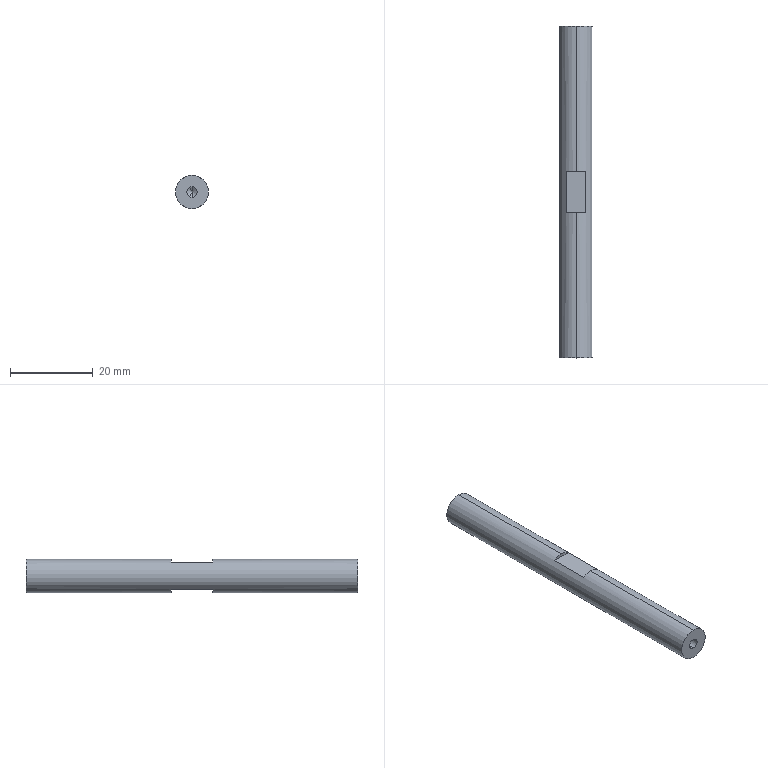Part | STEP file | PN_0039 | 1 solid | 18 faces | box 8 x 80 x 8 mm | volume 3898 mm3 | plane 8 | cylinder 6 | cone 4 | commonest cylinder face diameters 2.5 x4 8 x2
STEP:
#1=CARTESIAN_POINT('',(0.,0.,0.));
#2=DIRECTION('',(0.,0.,1.));
#3=DIRECTION('',(1.,0.,0.));
#4=AXIS2_PLACEMENT_3D('',#1,#2,#3);
#5=CARTESIAN_POINT('',(0.,32.5,1.25));
#6=VERTEX_POINT('',#5);
#7=CARTESIAN_POINT('',(0.,40.,1.25));
#8=VERTEX_POINT('',#7);
#9=CARTESIAN_POINT('',(0.,40.,1.25));
#10=DIRECTION('',(0.,1.,0.));
#11=VECTOR('',#10,1.);
#12=LINE('',#9,#11);
#13=CARTESIAN_POINT('',(0.,40.,0.));
#14=DIRECTION('',(0.,1.,0.));
#15=DIRECTION('',(0.,0.,1.));
#16=AXIS2_PLACEMENT_3D('',#13,#14,#15);
#17=CYLINDRICAL_SURFACE('',#16,1.25);
#18=CARTESIAN_POINT('',(6.283,0.));
#19=DIRECTION('',(0.,1.));
#20=VECTOR('',#19,1.);
#21=LINE('',#18,#20);
#22=(GEOMETRIC_REPRESENTATION_CONTEXT(2)PARAMETRIC_REPRESENTATION_CONTEXT()REPRESENTATION_CONTEXT('',''));
#23=DEFINITIONAL_REPRESENTATION('',(#21),#22);
#24=PCURVE('',#17,#23);
#25=CARTESIAN_POINT('',(0.,40.,0.));
#26=DIRECTION('',(0.,1.,0.));
#27=DIRECTION('',(0.,0.,1.));
#28=AXIS2_PLACEMENT_3D('',#25,#26,#27);
#29=CYLINDRICAL_SURFACE('',#28,1.25);
#30=CARTESIAN_POINT('',(0.,0.));
#31=DIRECTION('',(0.,1.));
#32=VECTOR('',#31,1.);
#33=LINE('',#30,#32);
#34=(GEOMETRIC_REPRESENTATION_CONTEXT(2)PARAMETRIC_REPRESENTATION_CONTEXT()REPRESENTATION_CONTEXT('',''));
#35=DEFINITIONAL_REPRESENTATION('',(#33),#34);
#36=PCURVE('',#29,#35);
#37=SURFACE_CURVE('',#12,(#24,#36),.PCURVE_S1.);
#38=EDGE_CURVE('',#6,#8,#37,.T.);
#39=ORIENTED_EDGE('',*,*,#38,.T.);
#40=CARTESIAN_POINT('',(0.,40.,-1.25));
#41=VERTEX_POINT('',#40);
#42=CARTESIAN_POINT('',(0.,40.,0.));
#43=DIRECTION('',(0.,1.,0.));
#44=DIRECTION('',(0.,0.,1.));
#45=AXIS2_PLACEMENT_3D('',#42,#43,#44);
#46=CIRCLE('',#45,1.25);
#47=CARTESIAN_POINT('',(0.,0.));
#48=DIRECTION('',(1.,0.));
#49=VECTOR('',#48,1.);
#50=LINE('',#47,#49);
#51=(GEOMETRIC_REPRESENTATION_CONTEXT(2)PARAMETRIC_REPRESENTATION_CONTEXT()REPRESENTATION_CONTEXT('',''));
#52=DEFINITIONAL_REPRESENTATION('',(#50),#51);
#53=PCURVE('',#17,#52);
#54=CARTESIAN_POINT('',(0.,40.,0.));
#55=DIRECTION('',(0.,1.,0.));
#56=DIRECTION('',(0.,0.,1.));
#57=AXIS2_PLACEMENT_3D('',#54,#55,#56);
#58=PLANE('',#57);
#59=CARTESIAN_POINT('',(0.,0.));
#60=DIRECTION('',(1.,0.));
#61=AXIS2_PLACEMENT_2D('',#59,#60);
#62=CIRCLE('',#61,1.25);
#63=(GEOMETRIC_REPRESENTATION_CONTEXT(2)PARAMETRIC_REPRESENTATION_CONTEXT()REPRESENTATION_CONTEXT('',''));
#64=DEFINITIONAL_REPRESENTATION('',(#62),#63);
#65=PCURVE('',#58,#64);
#66=SURFACE_CURVE('',#46,(#53,#65),.PCURVE_S1.);
#67=EDGE_CURVE('',#41,#8,#66,.T.);
#68=ORIENTED_EDGE('',*,*,#67,.F.);
#69=CARTESIAN_POINT('',(0.,32.5,-1.25));
#70=VERTEX_POINT('',#69);
#71=CARTESIAN_POINT('',(0.,40.,-1.25));
#72=DIRECTION('',(0.,1.,0.));
#73=VECTOR('',#72,1.);
#74=LINE('',#71,#73);
#75=CARTESIAN_POINT('',(3.142,0.));
#76=DIRECTION('',(0.,1.));
#77=VECTOR('',#76,1.);
#78=LINE('',#75,#77);
#79=(GEOMETRIC_REPRESENTATION_CONTEXT(2)PARAMETRIC_REPRESENTATION_CONTEXT()REPRESENTATION_CONTEXT('',''));
#80=DEFINITIONAL_REPRESENTATION('',(#78),#79);
#81=PCURVE('',#17,#80);
#82=CARTESIAN_POINT('',(3.142,0.));
#83=DIRECTION('',(0.,1.));
#84=VECTOR('',#83,1.);
#85=LINE('',#82,#84);
#86=(GEOMETRIC_REPRESENTATION_CONTEXT(2)PARAMETRIC_REPRESENTATION_CONTEXT()REPRESENTATION_CONTEXT('',''));
#87=DEFINITIONAL_REPRESENTATION('',(#85),#86);
#88=PCURVE('',#29,#87);
#89=SURFACE_CURVE('',#74,(#81,#88),.PCURVE_S1.);
#90=EDGE_CURVE('',#70,#41,#89,.T.);
#91=ORIENTED_EDGE('',*,*,#90,.F.);
#92=CARTESIAN_POINT('',(0.,32.5,0.));
#93=DIRECTION('',(0.,1.,0.));
#94=DIRECTION('',(0.,0.,1.));
#95=AXIS2_PLACEMENT_3D('',#92,#93,#94);
#96=CIRCLE('',#95,1.25);
#97=CARTESIAN_POINT('',(0.,-7.5));
#98=DIRECTION('',(1.,0.));
#99=VECTOR('',#98,1.);
#100=LINE('',#97,#99);
#101=(GEOMETRIC_REPRESENTATION_CONTEXT(2)PARAMETRIC_REPRESENTATION_CONTEXT()REPRESENTATION_CONTEXT('',''));
#102=DEFINITIONAL_REPRESENTATION('',(#100),#101);
#103=PCURVE('',#17,#102);
#104=CARTESIAN_POINT('',(0.,32.5,0.));
#105=DIRECTION('',(0.,1.,0.));
#106=DIRECTION('',(0.,0.,1.));
#107=AXIS2_PLACEMENT_3D('',#104,#105,#106);
#108=CONICAL_SURFACE('',#107,1.25,1.03);
#109=CARTESIAN_POINT('',(0.,0.));
#110=DIRECTION('',(1.,0.));
#111=VECTOR('',#110,1.);
#112=LINE('',#109,#111);
#113=(GEOMETRIC_REPRESENTATION_CONTEXT(2)PARAMETRIC_REPRESENTATION_CONTEXT()REPRESENTATION_CONTEXT('',''));
#114=DEFINITIONAL_REPRESENTATION('',(#112),#113);
#115=PCURVE('',#108,#114);
#116=SURFACE_CURVE('',#96,(#103,#115),.PCURVE_S1.);
#117=EDGE_CURVE('',#70,#6,#116,.T.);
#118=ORIENTED_EDGE('',*,*,#117,.T.);
#119=EDGE_LOOP('',(#39,#68,#91,#118));
#120=FACE_BOUND('',#119,.F.);
#121=ADVANCED_FACE('',(#120),#17,.F.);
#122=ORIENTED_EDGE('',*,*,#117,.F.);
#123=CARTESIAN_POINT('',(0.,31.749,0.));
#124=VERTEX_POINT('',#123);
#125=CARTESIAN_POINT('',(0.,32.5,-1.25));
#126=DIRECTION('',(0.,0.515,-0.8572));
#127=VECTOR('',#126,1.);
#128=LINE('',#125,#127);
#129=CARTESIAN_POINT('',(3.142,0.));
#130=DIRECTION('',(0.,1.));
#131=VECTOR('',#130,1.);
#132=LINE('',#129,#131);
#133=(GEOMETRIC_REPRESENTATION_CONTEXT(2)PARAMETRIC_REPRESENTATION_CONTEXT()REPRESENTATION_CONTEXT('',''));
#134=DEFINITIONAL_REPRESENTATION('',(#132),#133);
#135=PCURVE('',#108,#134);
#136=CARTESIAN_POINT('',(0.,32.5,0.));
#137=DIRECTION('',(0.,1.,0.));
#138=DIRECTION('',(0.,0.,1.));
#139=AXIS2_PLACEMENT_3D('',#136,#137,#138);
#140=CONICAL_SURFACE('',#139,1.25,1.03);
#141=CARTESIAN_POINT('',(3.142,0.));
#142=DIRECTION('',(0.,1.));
#143=VECTOR('',#142,1.);
#144=LINE('',#141,#143);
#145=(GEOMETRIC_REPRESENTATION_CONTEXT(2)PARAMETRIC_REPRESENTATION_CONTEXT()REPRESENTATION_CONTEXT('',''));
#146=DEFINITIONAL_REPRESENTATION('',(#144),#145);
#147=PCURVE('',#140,#146);
#148=SURFACE_CURVE('',#128,(#135,#147),.PCURVE_S1.);
#149=EDGE_CURVE('',#124,#70,#148,.T.);
#150=ORIENTED_EDGE('',*,*,#149,.F.);
#151=CARTESIAN_POINT('',(0.,32.5,1.25));
#152=DIRECTION('',(0.,0.515,0.8572));
#153=VECTOR('',#152,1.);
#154=LINE('',#151,#153);
#155=CARTESIAN_POINT('',(6.283,0.));
#156=DIRECTION('',(0.,1.));
#157=VECTOR('',#156,1.);
#158=LINE('',#155,#157);
#159=(GEOMETRIC_REPRESENTATION_CONTEXT(2)PARAMETRIC_REPRESENTATION_CONTEXT()REPRESENTATION_CONTEXT('',''));
#160=DEFINITIONAL_REPRESENTATION('',(#158),#159);
#161=PCURVE('',#108,#160);
#162=CARTESIAN_POINT('',(0.,0.));
#163=DIRECTION('',(0.,1.));
#164=VECTOR('',#163,1.);
#165=LINE('',#162,#164);
#166=(GEOMETRIC_REPRESENTATION_CONTEXT(2)PARAMETRIC_REPRESENTATION_CONTEXT()REPRESENTATION_CONTEXT('',''));
#167=DEFINITIONAL_REPRESENTATION('',(#165),#166);
#168=PCURVE('',#140,#167);
#169=SURFACE_CURVE('',#154,(#161,#168),.PCURVE_S1.);
#170=EDGE_CURVE('',#124,#6,#169,.T.);
#171=ORIENTED_EDGE('',*,*,#170,.T.);
#172=EDGE_LOOP('',(#122,#150,#171));
#173=FACE_BOUND('',#172,.F.);
#174=ADVANCED_FACE('',(#173),#108,.F.);
#175=CARTESIAN_POINT('',(0.,-32.5,-1.25));
#176=VERTEX_POINT('',#175);
#177=CARTESIAN_POINT('',(0.,-40.,-1.25));
#178=VERTEX_POINT('',#177);
#179=CARTESIAN_POINT('',(0.,-40.,-1.25));
#180=DIRECTION('',(0.,-1.,0.));
#181=VECTOR('',#180,1.);
#182=LINE('',#179,#181);
#183=CARTESIAN_POINT('',(0.,-40.,0.));
#184=DIRECTION('',(0.,-1.,0.));
#185=DIRECTION('',(0.,0.,-1.));
#186=AXIS2_PLACEMENT_3D('',#183,#184,#185);
#187=CYLINDRICAL_SURFACE('',#186,1.25);
#188=CARTESIAN_POINT('',(6.283,0.));
#189=DIRECTION('',(0.,1.));
#190=VECTOR('',#189,1.);
#191=LINE('',#188,#190);
#192=(GEOMETRIC_REPRESENTATION_CONTEXT(2)PARAMETRIC_REPRESENTATION_CONTEXT()REPRESENTATION_CONTEXT('',''));
#193=DEFINITIONAL_REPRESENTATION('',(#191),#192);
#194=PCURVE('',#187,#193);
#195=CARTESIAN_POINT('',(0.,-40.,0.));
#196=DIRECTION('',(0.,-1.,0.));
#197=DIRECTION('',(0.,0.,-1.));
#198=AXIS2_PLACEMENT_3D('',#195,#196,#197);
#199=CYLINDRICAL_SURFACE('',#198,1.25);
#200=CARTESIAN_POINT('',(0.,0.));
#201=DIRECTION('',(0.,1.));
#202=VECTOR('',#201,1.);
#203=LINE('',#200,#202);
#204=(GEOMETRIC_REPRESENTATION_CONTEXT(2)PARAMETRIC_REPRESENTATION_CONTEXT()REPRESENTATION_CONTEXT('',''));
#205=DEFINITIONAL_REPRESENTATION('',(#203),#204);
#206=PCURVE('',#199,#205);
#207=SURFACE_CURVE('',#182,(#194,#206),.PCURVE_S1.);
#208=EDGE_CURVE('',#176,#178,#207,.T.);
#209=ORIENTED_EDGE('',*,*,#208,.T.);
#210=CARTESIAN_POINT('',(0.,-40.,1.25));
#211=VERTEX_POINT('',#210);
#212=CARTESIAN_POINT('',(0.,-40.,0.));
#213=DIRECTION('',(0.,-1.,0.));
#214=DIRECTION('',(0.,0.,-1.));
#215=AXIS2_PLACEMENT_3D('',#212,#213,#214);
#216=CIRCLE('',#215,1.25);
#217=CARTESIAN_POINT('',(0.,0.));
#218=DIRECTION('',(1.,0.));
#219=VECTOR('',#218,1.);
#220=LINE('',#217,#219);
#221=(GEOMETRIC_REPRESENTATION_CONTEXT(2)PARAMETRIC_REPRESENTATION_CONTEXT()REPRESENTATION_CONTEXT('',''));
#222=DEFINITIONAL_REPRESENTATION('',(#220),#221);
#223=PCURVE('',#187,#222);
#224=CARTESIAN_POINT('',(0.,-40.,0.));
#225=DIRECTION('',(0.,1.,0.));
#226=DIRECTION('',(0.,0.,1.));
#227=AXIS2_PLACEMENT_3D('',#224,#225,#226);
#228=PLANE('',#227);
#229=CARTESIAN_POINT('',(-1.25,0.));
#230=CARTESIAN_POINT('',(-1.25,2.165));
#231=CARTESIAN_POINT('',(0.625,1.083));
#232=CARTESIAN_POINT('',(2.5,0.));
#233=CARTESIAN_POINT('',(0.625,-1.083));
#234=CARTESIAN_POINT('',(-1.25,-2.165));
#235=CARTESIAN_POINT('',(-1.25,0.));
#236=(BOUNDED_CURVE()B_SPLINE_CURVE(2,(#229,#230,#231,#232,#233,#234,#235),.UNSPECIFIED.,.T.,.F.)B_SPLINE_CURVE_WITH_KNOTS((1,2,2,2,2,1),(-2.094,0.,2.094,4.189,6.283,8.378),.UNSPECIFIED.)CURVE()GEOMETRIC_REPRESENTATION_ITEM()RATIONAL_B_SPLINE_CURVE((1.,0.5,1.,0.5,1.,0.5,1.))REPRESENTATION_ITEM(''));
#237=(GEOMETRIC_REPRESENTATION_CONTEXT(2)PARAMETRIC_REPRESENTATION_CONTEXT()REPRESENTATION_CONTEXT('',''));
#238=DEFINITIONAL_REPRESENTATION('',(#236),#237);
#239=PCURVE('',#228,#238);
#240=SURFACE_CURVE('',#216,(#223,#239),.PCURVE_S1.);
#241=EDGE_CURVE('',#211,#178,#240,.T.);
#242=ORIENTED_EDGE('',*,*,#241,.F.);
#243=CARTESIAN_POINT('',(0.,-32.5,1.25));
#244=VERTEX_POINT('',#243);
#245=CARTESIAN_POINT('',(0.,-40.,1.25));
#246=DIRECTION('',(0.,-1.,0.));
#247=VECTOR('',#246,1.);
#248=LINE('',#245,#247);
#249=CARTESIAN_POINT('',(3.142,0.));
#250=DIRECTION('',(0.,1.));
#251=VECTOR('',#250,1.);
#252=LINE('',#249,#251);
#253=(GEOMETRIC_REPRESENTATION_CONTEXT(2)PARAMETRIC_REPRESENTATION_CONTEXT()REPRESENTATION_CONTEXT('',''));
#254=DEFINITIONAL_REPRESENTATION('',(#252),#253);
#255=PCURVE('',#187,#254);
#256=CARTESIAN_POINT('',(3.142,0.));
#257=DIRECTION('',(0.,1.));
#258=VECTOR('',#257,1.);
#259=LINE('',#256,#258);
#260=(GEOMETRIC_REPRESENTATION_CONTEXT(2)PARAMETRIC_REPRESENTATION_CONTEXT()REPRESENTATION_CONTEXT('',''));
#261=DEFINITIONAL_REPRESENTATION('',(#259),#260);
#262=PCURVE('',#199,#261);
#263=SURFACE_CURVE('',#248,(#255,#262),.PCURVE_S1.);
#264=EDGE_CURVE('',#244,#211,#263,.T.);
#265=ORIENTED_EDGE('',*,*,#264,.F.);
#266=CARTESIAN_POINT('',(0.,-32.5,0.));
#267=DIRECTION('',(0.,-1.,0.));
#268=DIRECTION('',(0.,0.,-1.));
#269=AXIS2_PLACEMENT_3D('',#266,#267,#268);
#270=CIRCLE('',#269,1.25);
#271=CARTESIAN_POINT('',(0.,-7.5));
#272=DIRECTION('',(1.,0.));
#273=VECTOR('',#272,1.);
#274=LINE('',#271,#273);
#275=(GEOMETRIC_REPRESENTATION_CONTEXT(2)PARAMETRIC_REPRESENTATION_CONTEXT()REPRESENTATION_CONTEXT('',''));
#276=DEFINITIONAL_REPRESENTATION('',(#274),#275);
#277=PCURVE('',#187,#276);
#278=CARTESIAN_POINT('',(0.,-32.5,0.));
#279=DIRECTION('',(0.,-1.,0.));
#280=DIRECTION('',(0.,0.,-1.));
#281=AXIS2_PLACEMENT_3D('',#278,#279,#280);
#282=CONICAL_SURFACE('',#281,1.25,1.03);
#283=CARTESIAN_POINT('',(0.,0.));
#284=DIRECTION('',(1.,0.));
#285=VECTOR('',#284,1.);
#286=LINE('',#283,#285);
#287=(GEOMETRIC_REPRESENTATION_CONTEXT(2)PARAMETRIC_REPRESENTATION_CONTEXT()REPRESENTATION_CONTEXT('',''));
#288=DEFINITIONAL_REPRESENTATION('',(#286),#287);
#289=PCURVE('',#282,#288);
#290=SURFACE_CURVE('',#270,(#277,#289),.PCURVE_S1.);
#291=EDGE_CURVE('',#244,#176,#290,.T.);
#292=ORIENTED_EDGE('',*,*,#291,.T.);
#293=EDGE_LOOP('',(#209,#242,#265,#292));
#294=FACE_BOUND('',#293,.F.);
#295=ADVANCED_FACE('',(#294),#187,.F.);
#296=ORIENTED_EDGE('',*,*,#291,.F.);
#297=CARTESIAN_POINT('',(0.,-31.749,0.));
#298=VERTEX_POINT('',#297);
#299=CARTESIAN_POINT('',(0.,-32.5,1.25));
#300=DIRECTION('',(0.,-0.515,0.8572));
#301=VECTOR('',#300,1.);
#302=LINE('',#299,#301);
#303=CARTESIAN_POINT('',(3.142,0.));
#304=DIRECTION('',(0.,1.));
#305=VECTOR('',#304,1.);
#306=LINE('',#303,#305);
#307=(GEOMETRIC_REPRESENTATION_CONTEXT(2)PARAMETRIC_REPRESENTATION_CONTEXT()REPRESENTATION_CONTEXT('',''));
#308=DEFINITIONAL_REPRESENTATION('',(#306),#307);
#309=PCURVE('',#282,#308);
#310=CARTESIAN_POINT('',(0.,-32.5,0.));
#311=DIRECTION('',(0.,-1.,0.));
#312=DIRECTION('',(0.,0.,-1.));
#313=AXIS2_PLACEMENT_3D('',#310,#311,#312);
#314=CONICAL_SURFACE('',#313,1.25,1.03);
#315=CARTESIAN_POINT('',(3.142,0.));
#316=DIRECTION('',(0.,1.));
#317=VECTOR('',#316,1.);
#318=LINE('',#315,#317);
#319=(GEOMETRIC_REPRESENTATION_CONTEXT(2)PARAMETRIC_REPRESENTATION_CONTEXT()REPRESENTATION_CONTEXT('',''));
#320=DEFINITIONAL_REPRESENTATION('',(#318),#319);
#321=PCURVE('',#314,#320);
#322=SURFACE_CURVE('',#302,(#309,#321),.PCURVE_S1.);
#323=EDGE_CURVE('',#298,#244,#322,.T.);
#324=ORIENTED_EDGE('',*,*,#323,.F.);
#325=CARTESIAN_POINT('',(0.,-32.5,-1.25));
#326=DIRECTION('',(0.,-0.515,-0.8572));
#327=VECTOR('',#326,1.);
#328=LINE('',#325,#327);
#329=CARTESIAN_POINT('',(6.283,0.));
#330=DIRECTION('',(0.,1.));
#331=VECTOR('',#330,1.);
#332=LINE('',#329,#331);
#333=(GEOMETRIC_REPRESENTATION_CONTEXT(2)PARAMETRIC_REPRESENTATION_CONTEXT()REPRESENTATION_CONTEXT('',''));
#334=DEFINITIONAL_REPRESENTATION('',(#332),#333);
#335=PCURVE('',#282,#334);
#336=CARTESIAN_POINT('',(0.,0.));
#337=DIRECTION('',(0.,1.));
#338=VECTOR('',#337,1.);
#339=LINE('',#336,#338);
#340=(GEOMETRIC_REPRESENTATION_CONTEXT(2)PARAMETRIC_REPRESENTATION_CONTEXT()REPRESENTATION_CONTEXT('',''));
#341=DEFINITIONAL_REPRESENTATION('',(#339),#340);
#342=PCURVE('',#314,#341);
#343=SURFACE_CURVE('',#328,(#335,#342),.PCURVE_S1.);
#344=EDGE_CURVE('',#298,#176,#343,.T.);
#345=ORIENTED_EDGE('',*,*,#344,.T.);
#346=EDGE_LOOP('',(#296,#324,#345));
#347=FACE_BOUND('',#346,.F.);
#348=ADVANCED_FACE('',(#347),#282,.F.);
#349=CARTESIAN_POINT('',(0.,40.,4.));
#350=VERTEX_POINT('',#349);
#351=CARTESIAN_POINT('',(0.,40.,-4.));
#352=VERTEX_POINT('',#351);
#353=CARTESIAN_POINT('',(0.,40.,0.));
#354=DIRECTION('',(0.,1.,0.));
#355=DIRECTION('',(0.,0.,1.));
#356=AXIS2_PLACEMENT_3D('',#353,#354,#355);
#357=CIRCLE('',#356,4.);
#358=CARTESIAN_POINT('',(0.,40.,0.));
#359=DIRECTION('',(0.,-1.,0.));
#360=DIRECTION('',(0.,0.,-1.));
#361=AXIS2_PLACEMENT_3D('',#358,#359,#360);
#362=CYLINDRICAL_SURFACE('',#361,4.);
#363=CARTESIAN_POINT('',(3.142,0.));
#364=DIRECTION('',(-1.,0.));
#365=VECTOR('',#364,1.);
#366=LINE('',#363,#365);
#367=(GEOMETRIC_REPRESENTATION_CONTEXT(2)PARAMETRIC_REPRESENTATION_CONTEXT()REPRESENTATION_CONTEXT('',''));
#368=DEFINITIONAL_REPRESENTATION('',(#366),#367);
#369=PCURVE('',#362,#368);
#370=CARTESIAN_POINT('',(0.,0.));
#371=DIRECTION('',(1.,0.));
#372=AXIS2_PLACEMENT_2D('',#370,#371);
#373=CIRCLE('',#372,4.);
#374=(GEOMETRIC_REPRESENTATION_CONTEXT(2)PARAMETRIC_REPRESENTATION_CONTEXT()REPRESENTATION_CONTEXT('',''));
#375=DEFINITIONAL_REPRESENTATION('',(#373),#374);
#376=PCURVE('',#58,#375);
#377=SURFACE_CURVE('',#357,(#369,#376),.PCURVE_S1.);
#378=EDGE_CURVE('',#350,#352,#377,.T.);
#379=ORIENTED_EDGE('',*,*,#378,.F.);
#380=CARTESIAN_POINT('',(0.,5.,4.));
#381=VERTEX_POINT('',#380);
#382=CARTESIAN_POINT('',(0.,40.,4.));
#383=DIRECTION('',(0.,-1.,0.));
#384=VECTOR('',#383,1.);
#385=LINE('',#382,#384);
#386=CARTESIAN_POINT('',(3.142,0.));
#387=DIRECTION('',(0.,1.));
#388=VECTOR('',#387,1.);
#389=LINE('',#386,#388);
#390=(GEOMETRIC_REPRESENTATION_CONTEXT(2)PARAMETRIC_REPRESENTATION_CONTEXT()REPRESENTATION_CONTEXT('',''));
#391=DEFINITIONAL_REPRESENTATION('',(#389),#390);
#392=PCURVE('',#362,#391);
#393=CARTESIAN_POINT('',(0.,40.,0.));
#394=DIRECTION('',(0.,-1.,0.));
#395=DIRECTION('',(0.,0.,-1.));
#396=AXIS2_PLACEMENT_3D('',#393,#394,#395);
#397=CYLINDRICAL_SURFACE('',#396,4.);
#398=CARTESIAN_POINT('',(3.142,0.));
#399=DIRECTION('',(0.,1.));
#400=VECTOR('',#399,1.);
#401=LINE('',#398,#400);
#402=(GEOMETRIC_REPRESENTATION_CONTEXT(2)PARAMETRIC_REPRESENTATION_CONTEXT()REPRESENTATION_CONTEXT('',''));
#403=DEFINITIONAL_REPRESENTATION('',(#401),#402);
#404=PCURVE('',#397,#403);
#405=SURFACE_CURVE('',#385,(#392,#404),.PCURVE_S1.);
#406=EDGE_CURVE('',#350,#381,#405,.T.);
#407=ORIENTED_EDGE('',*,*,#406,.T.);
#408=CARTESIAN_POINT('',(2.332,5.,3.25));
#409=VERTEX_POINT('',#408);
#410=CARTESIAN_POINT('',(0.,5.,0.));
#411=DIRECTION('',(0.,1.,0.));
#412=DIRECTION('',(0.,0.,1.));
#413=AXIS2_PLACEMENT_3D('',#410,#411,#412);
#414=CIRCLE('',#413,4.);
#415=CARTESIAN_POINT('',(3.142,35.));
#416=DIRECTION('',(-1.,0.));
#417=VECTOR('',#416,1.);
#418=LINE('',#415,#417);
#419=(GEOMETRIC_REPRESENTATION_CONTEXT(2)PARAMETRIC_REPRESENTATION_CONTEXT()REPRESENTATION_CONTEXT('',''));
#420=DEFINITIONAL_REPRESENTATION('',(#418),#419);
#421=PCURVE('',#362,#420);
#422=CARTESIAN_POINT('',(0.,5.,0.));
#423=DIRECTION('',(0.,1.,0.));
#424=DIRECTION('',(0.,0.,1.));
#425=AXIS2_PLACEMENT_3D('',#422,#423,#424);
#426=PLANE('',#425);
#427=CARTESIAN_POINT('',(0.,0.));
#428=DIRECTION('',(1.,0.));
#429=AXIS2_PLACEMENT_2D('',#427,#428);
#430=CIRCLE('',#429,4.);
#431=(GEOMETRIC_REPRESENTATION_CONTEXT(2)PARAMETRIC_REPRESENTATION_CONTEXT()REPRESENTATION_CONTEXT('',''));
#432=DEFINITIONAL_REPRESENTATION('',(#430),#431);
#433=PCURVE('',#426,#432);
#434=SURFACE_CURVE('',#414,(#421,#433),.PCURVE_S1.);
#435=EDGE_CURVE('',#381,#409,#434,.T.);
#436=ORIENTED_EDGE('',*,*,#435,.T.);
#437=CARTESIAN_POINT('',(2.332,-5.,3.25));
#438=VERTEX_POINT('',#437);
#439=CARTESIAN_POINT('',(2.332,-5.,3.25));
#440=DIRECTION('',(0.,1.,0.));
#441=VECTOR('',#440,1.);
#442=LINE('',#439,#441);
#443=CARTESIAN_POINT('',(2.519,45.));
#444=DIRECTION('',(0.,-1.));
#445=VECTOR('',#444,1.);
#446=LINE('',#443,#445);
#447=(GEOMETRIC_REPRESENTATION_CONTEXT(2)PARAMETRIC_REPRESENTATION_CONTEXT()REPRESENTATION_CONTEXT('',''));
#448=DEFINITIONAL_REPRESENTATION('',(#446),#447);
#449=PCURVE('',#362,#448);
#450=CARTESIAN_POINT('',(-2.332,-5.,3.25));
#451=DIRECTION('',(0.,0.,-1.));
#452=DIRECTION('',(-1.,0.,0.));
#453=AXIS2_PLACEMENT_3D('',#450,#451,#452);
#454=PLANE('',#453);
#455=CARTESIAN_POINT('',(-4.664,0.));
#456=DIRECTION('',(0.,1.));
#457=VECTOR('',#456,1.);
#458=LINE('',#455,#457);
#459=(GEOMETRIC_REPRESENTATION_CONTEXT(2)PARAMETRIC_REPRESENTATION_CONTEXT()REPRESENTATION_CONTEXT('',''));
#460=DEFINITIONAL_REPRESENTATION('',(#458),#459);
#461=PCURVE('',#454,#460);
#462=SURFACE_CURVE('',#442,(#449,#461),.PCURVE_S1.);
#463=EDGE_CURVE('',#438,#409,#462,.T.);
#464=ORIENTED_EDGE('',*,*,#463,.F.);
#465=CARTESIAN_POINT('',(0.,-5.,4.));
#466=VERTEX_POINT('',#465);
#467=CARTESIAN_POINT('',(0.,-5.,0.));
#468=DIRECTION('',(0.,1.,0.));
#469=DIRECTION('',(0.,0.,1.));
#470=AXIS2_PLACEMENT_3D('',#467,#468,#469);
#471=CIRCLE('',#470,4.);
#472=CARTESIAN_POINT('',(3.142,45.));
#473=DIRECTION('',(-1.,0.));
#474=VECTOR('',#473,1.);
#475=LINE('',#472,#474);
#476=(GEOMETRIC_REPRESENTATION_CONTEXT(2)PARAMETRIC_REPRESENTATION_CONTEXT()REPRESENTATION_CONTEXT('',''));
#477=DEFINITIONAL_REPRESENTATION('',(#475),#476);
#478=PCURVE('',#362,#477);
#479=CARTESIAN_POINT('',(0.,-5.,0.));
#480=DIRECTION('',(0.,1.,0.));
#481=DIRECTION('',(0.,0.,1.));
#482=AXIS2_PLACEMENT_3D('',#479,#480,#481);
#483=PLANE('',#482);
#484=CARTESIAN_POINT('',(0.,0.));
#485=DIRECTION('',(1.,0.));
#486=AXIS2_PLACEMENT_2D('',#484,#485);
#487=CIRCLE('',#486,4.);
#488=(GEOMETRIC_REPRESENTATION_CONTEXT(2)PARAMETRIC_REPRESENTATION_CONTEXT()REPRESENTATION_CONTEXT('',''));
#489=DEFINITIONAL_REPRESENTATION('',(#487),#488);
#490=PCURVE('',#483,#489);
#491=SURFACE_CURVE('',#471,(#478,#490),.PCURVE_S1.);
#492=EDGE_CURVE('',#466,#438,#491,.T.);
#493=ORIENTED_EDGE('',*,*,#492,.F.);
#494=CARTESIAN_POINT('',(0.,-40.,4.));
#495=VERTEX_POINT('',#494);
#496=CARTESIAN_POINT('',(0.,40.,4.));
#497=DIRECTION('',(0.,-1.,0.));
#498=VECTOR('',#497,1.);
#499=LINE('',#496,#498);
#500=CARTESIAN_POINT('',(3.142,0.));
#501=DIRECTION('',(0.,1.));
#502=VECTOR('',#501,1.);
#503=LINE('',#500,#502);
#504=(GEOMETRIC_REPRESENTATION_CONTEXT(2)PARAMETRIC_REPRESENTATION_CONTEXT()REPRESENTATION_CONTEXT('',''));
#505=DEFINITIONAL_REPRESENTATION('',(#503),#504);
#506=PCURVE('',#362,#505);
#507=CARTESIAN_POINT('',(3.142,0.));
#508=DIRECTION('',(0.,1.));
#509=VECTOR('',#508,1.);
#510=LINE('',#507,#509);
#511=(GEOMETRIC_REPRESENTATION_CONTEXT(2)PARAMETRIC_REPRESENTATION_CONTEXT()REPRESENTATION_CONTEXT('',''));
#512=DEFINITIONAL_REPRESENTATION('',(#510),#511);
#513=PCURVE('',#397,#512);
#514=SURFACE_CURVE('',#499,(#506,#513),.PCURVE_S1.);
#515=EDGE_CURVE('',#466,#495,#514,.T.);
#516=ORIENTED_EDGE('',*,*,#515,.T.);
#517=CARTESIAN_POINT('',(0.,-40.,-4.));
#518=VERTEX_POINT('',#517);
#519=CARTESIAN_POINT('',(0.,-40.,0.));
#520=DIRECTION('',(0.,1.,0.));
#521=DIRECTION('',(0.,0.,1.));
#522=AXIS2_PLACEMENT_3D('',#519,#520,#521);
#523=CIRCLE('',#522,4.);
#524=CARTESIAN_POINT('',(3.142,80.));
#525=DIRECTION('',(-1.,0.));
#526=VECTOR('',#525,1.);
#527=LINE('',#524,#526);
#528=(GEOMETRIC_REPRESENTATION_CONTEXT(2)PARAMETRIC_REPRESENTATION_CONTEXT()REPRESENTATION_CONTEXT('',''));
#529=DEFINITIONAL_REPRESENTATION('',(#527),#528);
#530=PCURVE('',#362,#529);
#531=CARTESIAN_POINT('',(0.,0.));
#532=DIRECTION('',(1.,0.));
#533=AXIS2_PLACEMENT_2D('',#531,#532);
#534=CIRCLE('',#533,4.);
#535=(GEOMETRIC_REPRESENTATION_CONTEXT(2)PARAMETRIC_REPRESENTATION_CONTEXT()REPRESENTATION_CONTEXT('',''));
#536=DEFINITIONAL_REPRESENTATION('',(#534),#535);
#537=PCURVE('',#228,#536);
#538=SURFACE_CURVE('',#523,(#530,#537),.PCURVE_S1.);
#539=EDGE_CURVE('',#495,#518,#538,.T.);
#540=ORIENTED_EDGE('',*,*,#539,.T.);
#541=CARTESIAN_POINT('',(0.,-5.,-4.));
#542=VERTEX_POINT('',#541);
#543=CARTESIAN_POINT('',(0.,40.,-4.));
#544=DIRECTION('',(0.,-1.,0.));
#545=VECTOR('',#544,1.);
#546=LINE('',#543,#545);
#547=CARTESIAN_POINT('',(0.,0.));
#548=DIRECTION('',(0.,1.));
#549=VECTOR('',#548,1.);
#550=LINE('',#547,#549);
#551=(GEOMETRIC_REPRESENTATION_CONTEXT(2)PARAMETRIC_REPRESENTATION_CONTEXT()REPRESENTATION_CONTEXT('',''));
#552=DEFINITIONAL_REPRESENTATION('',(#550),#551);
#553=PCURVE('',#362,#552);
#554=CARTESIAN_POINT('',(6.283,0.));
#555=DIRECTION('',(0.,1.));
#556=VECTOR('',#555,1.);
#557=LINE('',#554,#556);
#558=(GEOMETRIC_REPRESENTATION_CONTEXT(2)PARAMETRIC_REPRESENTATION_CONTEXT()REPRESENTATION_CONTEXT('',''));
#559=DEFINITIONAL_REPRESENTATION('',(#557),#558);
#560=PCURVE('',#397,#559);
#561=SURFACE_CURVE('',#546,(#553,#560),.PCURVE_S1.);
#562=EDGE_CURVE('',#542,#518,#561,.T.);
#563=ORIENTED_EDGE('',*,*,#562,.F.);
#564=CARTESIAN_POINT('',(2.332,-5.,-3.25));
#565=VERTEX_POINT('',#564);
#566=CARTESIAN_POINT('',(0.,-5.,0.));
#567=DIRECTION('',(0.,1.,0.));
#568=DIRECTION('',(0.,0.,1.));
#569=AXIS2_PLACEMENT_3D('',#566,#567,#568);
#570=CIRCLE('',#569,4.);
#571=CARTESIAN_POINT('',(3.142,45.));
#572=DIRECTION('',(-1.,0.));
#573=VECTOR('',#572,1.);
#574=LINE('',#571,#573);
#575=(GEOMETRIC_REPRESENTATION_CONTEXT(2)PARAMETRIC_REPRESENTATION_CONTEXT()REPRESENTATION_CONTEXT('',''));
#576=DEFINITIONAL_REPRESENTATION('',(#574),#575);
#577=PCURVE('',#362,#576);
#578=CARTESIAN_POINT('',(0.,-5.,0.));
#579=DIRECTION('',(0.,1.,0.));
#580=DIRECTION('',(0.,0.,1.));
#581=AXIS2_PLACEMENT_3D('',#578,#579,#580);
#582=PLANE('',#581);
#583=CARTESIAN_POINT('',(0.,0.));
#584=DIRECTION('',(1.,0.));
#585=AXIS2_PLACEMENT_2D('',#583,#584);
#586=CIRCLE('',#585,4.);
#587=(GEOMETRIC_REPRESENTATION_CONTEXT(2)PARAMETRIC_REPRESENTATION_CONTEXT()REPRESENTATION_CONTEXT('',''));
#588=DEFINITIONAL_REPRESENTATION('',(#586),#587);
#589=PCURVE('',#582,#588);
#590=SURFACE_CURVE('',#570,(#577,#589),.PCURVE_S1.);
#591=EDGE_CURVE('',#565,#542,#590,.T.);
#592=ORIENTED_EDGE('',*,*,#591,.F.);
#593=CARTESIAN_POINT('',(2.332,5.,-3.25));
#594=VERTEX_POINT('',#593);
#595=CARTESIAN_POINT('',(2.332,-5.,-3.25));
#596=DIRECTION('',(0.,1.,0.));
#597=VECTOR('',#596,1.);
#598=LINE('',#595,#597);
#599=CARTESIAN_POINT('',(0.6224,45.));
#600=DIRECTION('',(0.,-1.));
#601=VECTOR('',#600,1.);
#602=LINE('',#599,#601);
#603=(GEOMETRIC_REPRESENTATION_CONTEXT(2)PARAMETRIC_REPRESENTATION_CONTEXT()REPRESENTATION_CONTEXT('',''));
#604=DEFINITIONAL_REPRESENTATION('',(#602),#603);
#605=PCURVE('',#362,#604);
#606=CARTESIAN_POINT('',(2.332,-5.,-3.25));
#607=DIRECTION('',(0.,0.,1.));
#608=DIRECTION('',(1.,0.,0.));
#609=AXIS2_PLACEMENT_3D('',#606,#607,#608);
#610=PLANE('',#609);
#611=CARTESIAN_POINT('',(0.,0.));
#612=DIRECTION('',(0.,1.));
#613=VECTOR('',#612,1.);
#614=LINE('',#611,#613);
#615=(GEOMETRIC_REPRESENTATION_CONTEXT(2)PARAMETRIC_REPRESENTATION_CONTEXT()REPRESENTATION_CONTEXT('',''));
#616=DEFINITIONAL_REPRESENTATION('',(#614),#615);
#617=PCURVE('',#610,#616);
#618=SURFACE_CURVE('',#598,(#605,#617),.PCURVE_S1.);
#619=EDGE_CURVE('',#565,#594,#618,.T.);
#620=ORIENTED_EDGE('',*,*,#619,.T.);
#621=CARTESIAN_POINT('',(0.,5.,-4.));
#622=VERTEX_POINT('',#621);
#623=CARTESIAN_POINT('',(0.,5.,0.));
#624=DIRECTION('',(0.,1.,0.));
#625=DIRECTION('',(0.,0.,1.));
#626=AXIS2_PLACEMENT_3D('',#623,#624,#625);
#627=CIRCLE('',#626,4.);
#628=CARTESIAN_POINT('',(3.142,35.));
#629=DIRECTION('',(-1.,0.));
#630=VECTOR('',#629,1.);
#631=LINE('',#628,#630);
#632=(GEOMETRIC_REPRESENTATION_CONTEXT(2)PARAMETRIC_REPRESENTATION_CONTEXT()REPRESENTATION_CONTEXT('',''));
#633=DEFINITIONAL_REPRESENTATION('',(#631),#632);
#634=PCURVE('',#362,#633);
#635=CARTESIAN_POINT('',(0.,5.,0.));
#636=DIRECTION('',(0.,1.,0.));
#637=DIRECTION('',(0.,0.,1.));
#638=AXIS2_PLACEMENT_3D('',#635,#636,#637);
#639=PLANE('',#638);
#640=CARTESIAN_POINT('',(0.,0.));
#641=DIRECTION('',(1.,0.));
#642=AXIS2_PLACEMENT_2D('',#640,#641);
#643=CIRCLE('',#642,4.);
#644=(GEOMETRIC_REPRESENTATION_CONTEXT(2)PARAMETRIC_REPRESENTATION_CONTEXT()REPRESENTATION_CONTEXT('',''));
#645=DEFINITIONAL_REPRESENTATION('',(#643),#644);
#646=PCURVE('',#639,#645);
#647=SURFACE_CURVE('',#627,(#634,#646),.PCURVE_S1.);
#648=EDGE_CURVE('',#594,#622,#647,.T.);
#649=ORIENTED_EDGE('',*,*,#648,.T.);
#650=CARTESIAN_POINT('',(0.,40.,-4.));
#651=DIRECTION('',(0.,-1.,0.));
#652=VECTOR('',#651,1.);
#653=LINE('',#650,#652);
#654=CARTESIAN_POINT('',(0.,0.));
#655=DIRECTION('',(0.,1.));
#656=VECTOR('',#655,1.);
#657=LINE('',#654,#656);
#658=(GEOMETRIC_REPRESENTATION_CONTEXT(2)PARAMETRIC_REPRESENTATION_CONTEXT()REPRESENTATION_CONTEXT('',''));
#659=DEFINITIONAL_REPRESENTATION('',(#657),#658);
#660=PCURVE('',#362,#659);
#661=CARTESIAN_POINT('',(6.283,0.));
#662=DIRECTION('',(0.,1.));
#663=VECTOR('',#662,1.);
#664=LINE('',#661,#663);
#665=(GEOMETRIC_REPRESENTATION_CONTEXT(2)PARAMETRIC_REPRESENTATION_CONTEXT()REPRESENTATION_CONTEXT('',''));
#666=DEFINITIONAL_REPRESENTATION('',(#664),#665);
#667=PCURVE('',#397,#666);
#668=SURFACE_CURVE('',#653,(#660,#667),.PCURVE_S1.);
#669=EDGE_CURVE('',#352,#622,#668,.T.);
#670=ORIENTED_EDGE('',*,*,#669,.F.);
#671=EDGE_LOOP('',(#379,#407,#436,#464,#493,#516,#540,#563,#592,#620,#649,#670));
#672=FACE_BOUND('',#671,.T.);
#673=ADVANCED_FACE('',(#672),#362,.T.);
#674=ORIENTED_EDGE('',*,*,#406,.F.);
#675=CARTESIAN_POINT('',(0.,40.,0.));
#676=DIRECTION('',(0.,1.,0.));
#677=DIRECTION('',(0.,0.,1.));
#678=AXIS2_PLACEMENT_3D('',#675,#676,#677);
#679=CIRCLE('',#678,4.);
#680=CARTESIAN_POINT('',(9.425,0.));
#681=DIRECTION('',(-1.,0.));
#682=VECTOR('',#681,1.);
#683=LINE('',#680,#682);
#684=(GEOMETRIC_REPRESENTATION_CONTEXT(2)PARAMETRIC_REPRESENTATION_CONTEXT()REPRESENTATION_CONTEXT('',''));
#685=DEFINITIONAL_REPRESENTATION('',(#683),#684);
#686=PCURVE('',#397,#685);
#687=CARTESIAN_POINT('',(0.,0.));
#688=DIRECTION('',(1.,0.));
#689=AXIS2_PLACEMENT_2D('',#687,#688);
#690=CIRCLE('',#689,4.);
#691=(GEOMETRIC_REPRESENTATION_CONTEXT(2)PARAMETRIC_REPRESENTATION_CONTEXT()REPRESENTATION_CONTEXT('',''));
#692=DEFINITIONAL_REPRESENTATION('',(#690),#691);
#693=PCURVE('',#58,#692);
#694=SURFACE_CURVE('',#679,(#686,#693),.PCURVE_S1.);
#695=EDGE_CURVE('',#352,#350,#694,.T.);
#696=ORIENTED_EDGE('',*,*,#695,.F.);
#697=ORIENTED_EDGE('',*,*,#669,.T.);
#698=CARTESIAN_POINT('',(-2.332,5.,-3.25));
#699=VERTEX_POINT('',#698);
#700=CARTESIAN_POINT('',(0.,5.,0.));
#701=DIRECTION('',(0.,1.,0.));
#702=DIRECTION('',(0.,0.,1.));
#703=AXIS2_PLACEMENT_3D('',#700,#701,#702);
#704=CIRCLE('',#703,4.);
#705=CARTESIAN_POINT('',(9.425,35.));
#706=DIRECTION('',(-1.,0.));
#707=VECTOR('',#706,1.);
#708=LINE('',#705,#707);
#709=(GEOMETRIC_REPRESENTATION_CONTEXT(2)PARAMETRIC_REPRESENTATION_CONTEXT()REPRESENTATION_CONTEXT('',''));
#710=DEFINITIONAL_REPRESENTATION('',(#708),#709);
#711=PCURVE('',#397,#710);
#712=CARTESIAN_POINT('',(0.,0.));
#713=DIRECTION('',(1.,0.));
#714=AXIS2_PLACEMENT_2D('',#712,#713);
#715=CIRCLE('',#714,4.);
#716=(GEOMETRIC_REPRESENTATION_CONTEXT(2)PARAMETRIC_REPRESENTATION_CONTEXT()REPRESENTATION_CONTEXT('',''));
#717=DEFINITIONAL_REPRESENTATION('',(#715),#716);
#718=PCURVE('',#639,#717);
#719=SURFACE_CURVE('',#704,(#711,#718),.PCURVE_S1.);
#720=EDGE_CURVE('',#622,#699,#719,.T.);
#721=ORIENTED_EDGE('',*,*,#720,.T.);
#722=CARTESIAN_POINT('',(-2.332,-5.,-3.25));
#723=VERTEX_POINT('',#722);
#724=CARTESIAN_POINT('',(-2.332,-5.,-3.25));
#725=DIRECTION('',(0.,1.,0.));
#726=VECTOR('',#725,1.);
#727=LINE('',#724,#726);
#728=CARTESIAN_POINT('',(5.661,45.));
#729=DIRECTION('',(0.,-1.));
#730=VECTOR('',#729,1.);
#731=LINE('',#728,#730);
#732=(GEOMETRIC_REPRESENTATION_CONTEXT(2)PARAMETRIC_REPRESENTATION_CONTEXT()REPRESENTATION_CONTEXT('',''));
#733=DEFINITIONAL_REPRESENTATION('',(#731),#732);
#734=PCURVE('',#397,#733);
#735=CARTESIAN_POINT('',(-4.664,0.));
#736=DIRECTION('',(0.,1.));
#737=VECTOR('',#736,1.);
#738=LINE('',#735,#737);
#739=(GEOMETRIC_REPRESENTATION_CONTEXT(2)PARAMETRIC_REPRESENTATION_CONTEXT()REPRESENTATION_CONTEXT('',''));
#740=DEFINITIONAL_REPRESENTATION('',(#738),#739);
#741=PCURVE('',#610,#740);
#742=SURFACE_CURVE('',#727,(#734,#741),.PCURVE_S1.);
#743=EDGE_CURVE('',#723,#699,#742,.T.);
#744=ORIENTED_EDGE('',*,*,#743,.F.);
#745=CARTESIAN_POINT('',(0.,-5.,0.));
#746=DIRECTION('',(0.,1.,0.));
#747=DIRECTION('',(0.,0.,1.));
#748=AXIS2_PLACEMENT_3D('',#745,#746,#747);
#749=CIRCLE('',#748,4.);
#750=CARTESIAN_POINT('',(9.425,45.));
#751=DIRECTION('',(-1.,0.));
#752=VECTOR('',#751,1.);
#753=LINE('',#750,#752);
#754=(GEOMETRIC_REPRESENTATION_CONTEXT(2)PARAMETRIC_REPRESENTATION_CONTEXT()REPRESENTATION_CONTEXT('',''));
#755=DEFINITIONAL_REPRESENTATION('',(#753),#754);
#756=PCURVE('',#397,#755);
#757=CARTESIAN_POINT('',(0.,0.));
#758=DIRECTION('',(1.,0.));
#759=AXIS2_PLACEMENT_2D('',#757,#758);
#760=CIRCLE('',#759,4.);
#761=(GEOMETRIC_REPRESENTATION_CONTEXT(2)PARAMETRIC_REPRESENTATION_CONTEXT()REPRESENTATION_CONTEXT('',''));
#762=DEFINITIONAL_REPRESENTATION('',(#760),#761);
#763=PCURVE('',#582,#762);
#764=SURFACE_CURVE('',#749,(#756,#763),.PCURVE_S1.);
#765=EDGE_CURVE('',#542,#723,#764,.T.);
#766=ORIENTED_EDGE('',*,*,#765,.F.);
#767=ORIENTED_EDGE('',*,*,#562,.T.);
#768=CARTESIAN_POINT('',(0.,-40.,0.));
#769=DIRECTION('',(0.,1.,0.));
#770=DIRECTION('',(0.,0.,1.));
#771=AXIS2_PLACEMENT_3D('',#768,#769,#770);
#772=CIRCLE('',#771,4.);
#773=CARTESIAN_POINT('',(9.425,80.));
#774=DIRECTION('',(-1.,0.));
#775=VECTOR('',#774,1.);
#776=LINE('',#773,#775);
#777=(GEOMETRIC_REPRESENTATION_CONTEXT(2)PARAMETRIC_REPRESENTATION_CONTEXT()REPRESENTATION_CONTEXT('',''));
#778=DEFINITIONAL_REPRESENTATION('',(#776),#777);
#779=PCURVE('',#397,#778);
#780=CARTESIAN_POINT('',(0.,0.));
#781=DIRECTION('',(1.,0.));
#782=AXIS2_PLACEMENT_2D('',#780,#781);
#783=CIRCLE('',#782,4.);
#784=(GEOMETRIC_REPRESENTATION_CONTEXT(2)PARAMETRIC_REPRESENTATION_CONTEXT()REPRESENTATION_CONTEXT('',''));
#785=DEFINITIONAL_REPRESENTATION('',(#783),#784);
#786=PCURVE('',#228,#785);
#787=SURFACE_CURVE('',#772,(#779,#786),.PCURVE_S1.);
#788=EDGE_CURVE('',#518,#495,#787,.T.);
#789=ORIENTED_EDGE('',*,*,#788,.T.);
#790=ORIENTED_EDGE('',*,*,#515,.F.);
#791=CARTESIAN_POINT('',(-2.332,-5.,3.25));
#792=VERTEX_POINT('',#791);
#793=CARTESIAN_POINT('',(0.,-5.,0.));
#794=DIRECTION('',(0.,1.,0.));
#795=DIRECTION('',(0.,0.,1.));
#796=AXIS2_PLACEMENT_3D('',#793,#794,#795);
#797=CIRCLE('',#796,4.);
#798=CARTESIAN_POINT('',(9.425,45.));
#799=DIRECTION('',(-1.,0.));
#800=VECTOR('',#799,1.);
#801=LINE('',#798,#800);
#802=(GEOMETRIC_REPRESENTATION_CONTEXT(2)PARAMETRIC_REPRESENTATION_CONTEXT()REPRESENTATION_CONTEXT('',''));
#803=DEFINITIONAL_REPRESENTATION('',(#801),#802);
#804=PCURVE('',#397,#803);
#805=CARTESIAN_POINT('',(0.,0.));
#806=DIRECTION('',(1.,0.));
#807=AXIS2_PLACEMENT_2D('',#805,#806);
#808=CIRCLE('',#807,4.);
#809=(GEOMETRIC_REPRESENTATION_CONTEXT(2)PARAMETRIC_REPRESENTATION_CONTEXT()REPRESENTATION_CONTEXT('',''));
#810=DEFINITIONAL_REPRESENTATION('',(#808),#809);
#811=PCURVE('',#483,#810);
#812=SURFACE_CURVE('',#797,(#804,#811),.PCURVE_S1.);
#813=EDGE_CURVE('',#792,#466,#812,.T.);
#814=ORIENTED_EDGE('',*,*,#813,.F.);
#815=CARTESIAN_POINT('',(-2.332,5.,3.25));
#816=VERTEX_POINT('',#815);
#817=CARTESIAN_POINT('',(-2.332,-5.,3.25));
#818=DIRECTION('',(0.,1.,0.));
#819=VECTOR('',#818,1.);
#820=LINE('',#817,#819);
#821=CARTESIAN_POINT('',(3.764,45.));
#822=DIRECTION('',(0.,-1.));
#823=VECTOR('',#822,1.);
#824=LINE('',#821,#823);
#825=(GEOMETRIC_REPRESENTATION_CONTEXT(2)PARAMETRIC_REPRESENTATION_CONTEXT()REPRESENTATION_CONTEXT('',''));
#826=DEFINITIONAL_REPRESENTATION('',(#824),#825);
#827=PCURVE('',#397,#826);
#828=CARTESIAN_POINT('',(0.,0.));
#829=DIRECTION('',(0.,1.));
#830=VECTOR('',#829,1.);
#831=LINE('',#828,#830);
#832=(GEOMETRIC_REPRESENTATION_CONTEXT(2)PARAMETRIC_REPRESENTATION_CONTEXT()REPRESENTATION_CONTEXT('',''));
#833=DEFINITIONAL_REPRESENTATION('',(#831),#832);
#834=PCURVE('',#454,#833);
#835=SURFACE_CURVE('',#820,(#827,#834),.PCURVE_S1.);
#836=EDGE_CURVE('',#792,#816,#835,.T.);
#837=ORIENTED_EDGE('',*,*,#836,.T.);
#838=CARTESIAN_POINT('',(0.,5.,0.));
#839=DIRECTION('',(0.,1.,0.));
#840=DIRECTION('',(0.,0.,1.));
#841=AXIS2_PLACEMENT_3D('',#838,#839,#840);
#842=CIRCLE('',#841,4.);
#843=CARTESIAN_POINT('',(9.425,35.));
#844=DIRECTION('',(-1.,0.));
#845=VECTOR('',#844,1.);
#846=LINE('',#843,#845);
#847=(GEOMETRIC_REPRESENTATION_CONTEXT(2)PARAMETRIC_REPRESENTATION_CONTEXT()REPRESENTATION_CONTEXT('',''));
#848=DEFINITIONAL_REPRESENTATION('',(#846),#847);
#849=PCURVE('',#397,#848);
#850=CARTESIAN_POINT('',(0.,0.));
#851=DIRECTION('',(1.,0.));
#852=AXIS2_PLACEMENT_2D('',#850,#851);
#853=CIRCLE('',#852,4.);
#854=(GEOMETRIC_REPRESENTATION_CONTEXT(2)PARAMETRIC_REPRESENTATION_CONTEXT()REPRESENTATION_CONTEXT('',''));
#855=DEFINITIONAL_REPRESENTATION('',(#853),#854);
#856=PCURVE('',#426,#855);
#857=SURFACE_CURVE('',#842,(#849,#856),.PCURVE_S1.);
#858=EDGE_CURVE('',#816,#381,#857,.T.);
#859=ORIENTED_EDGE('',*,*,#858,.T.);
#860=EDGE_LOOP('',(#674,#696,#697,#721,#744,#766,#767,#789,#790,#814,#837,#859));
#861=FACE_BOUND('',#860,.T.);
#862=ADVANCED_FACE('',(#861),#397,.T.);
#863=CARTESIAN_POINT('',(0.,40.,0.));
#864=DIRECTION('',(0.,1.,0.));
#865=DIRECTION('',(0.,0.,1.));
#866=AXIS2_PLACEMENT_3D('',#863,#864,#865);
#867=CIRCLE('',#866,1.25);
#868=CARTESIAN_POINT('',(0.,0.));
#869=DIRECTION('',(1.,0.));
#870=AXIS2_PLACEMENT_2D('',#868,#869);
#871=CIRCLE('',#870,1.25);
#872=(GEOMETRIC_REPRESENTATION_CONTEXT(2)PARAMETRIC_REPRESENTATION_CONTEXT()REPRESENTATION_CONTEXT('',''));
#873=DEFINITIONAL_REPRESENTATION('',(#871),#872);
#874=PCURVE('',#58,#873);
#875=CARTESIAN_POINT('',(0.,0.));
#876=DIRECTION('',(1.,0.));
#877=VECTOR('',#876,1.);
#878=LINE('',#875,#877);
#879=(GEOMETRIC_REPRESENTATION_CONTEXT(2)PARAMETRIC_REPRESENTATION_CONTEXT()REPRESENTATION_CONTEXT('',''));
#880=DEFINITIONAL_REPRESENTATION('',(#878),#879);
#881=PCURVE('',#29,#880);
#882=SURFACE_CURVE('',#867,(#874,#881),.PCURVE_S1.);
#883=EDGE_CURVE('',#8,#41,#882,.T.);
#884=ORIENTED_EDGE('',*,*,#883,.F.);
#885=ORIENTED_EDGE('',*,*,#67,.F.);
#886=EDGE_LOOP('',(#884,#885));
#887=FACE_BOUND('',#886,.T.);
#888=ORIENTED_EDGE('',*,*,#695,.T.);
#889=ORIENTED_EDGE('',*,*,#378,.T.);
#890=EDGE_LOOP('',(#888,#889));
#891=FACE_BOUND('',#890,.T.);
#892=ADVANCED_FACE('',(#887,#891),#58,.T.);
#893=CARTESIAN_POINT('',(0.,-40.,0.));
#894=DIRECTION('',(0.,-1.,0.));
#895=DIRECTION('',(0.,0.,-1.));
#896=AXIS2_PLACEMENT_3D('',#893,#894,#895);
#897=CIRCLE('',#896,1.25);
#898=CARTESIAN_POINT('',(-1.25,0.));
#899=CARTESIAN_POINT('',(-1.25,2.165));
#900=CARTESIAN_POINT('',(0.625,1.083));
#901=CARTESIAN_POINT('',(2.5,0.));
#902=CARTESIAN_POINT('',(0.625,-1.083));
#903=CARTESIAN_POINT('',(-1.25,-2.165));
#904=CARTESIAN_POINT('',(-1.25,0.));
#905=(BOUNDED_CURVE()B_SPLINE_CURVE(2,(#898,#899,#900,#901,#902,#903,#904),.UNSPECIFIED.,.T.,.F.)B_SPLINE_CURVE_WITH_KNOTS((1,2,2,2,2,1),(-2.094,0.,2.094,4.189,6.283,8.378),.UNSPECIFIED.)CURVE()GEOMETRIC_REPRESENTATION_ITEM()RATIONAL_B_SPLINE_CURVE((1.,0.5,1.,0.5,1.,0.5,1.))REPRESENTATION_ITEM(''));
#906=(GEOMETRIC_REPRESENTATION_CONTEXT(2)PARAMETRIC_REPRESENTATION_CONTEXT()REPRESENTATION_CONTEXT('',''));
#907=DEFINITIONAL_REPRESENTATION('',(#905),#906);
#908=PCURVE('',#228,#907);
#909=CARTESIAN_POINT('',(0.,0.));
#910=DIRECTION('',(1.,0.));
#911=VECTOR('',#910,1.);
#912=LINE('',#909,#911);
#913=(GEOMETRIC_REPRESENTATION_CONTEXT(2)PARAMETRIC_REPRESENTATION_CONTEXT()REPRESENTATION_CONTEXT('',''));
#914=DEFINITIONAL_REPRESENTATION('',(#912),#913);
#915=PCURVE('',#199,#914);
#916=SURFACE_CURVE('',#897,(#908,#915),.PCURVE_S1.);
#917=EDGE_CURVE('',#178,#211,#916,.T.);
#918=ORIENTED_EDGE('',*,*,#917,.F.);
#919=ORIENTED_EDGE('',*,*,#241,.F.);
#920=EDGE_LOOP('',(#918,#919));
#921=FACE_BOUND('',#920,.T.);
#922=ORIENTED_EDGE('',*,*,#788,.F.);
#923=ORIENTED_EDGE('',*,*,#539,.F.);
#924=EDGE_LOOP('',(#922,#923));
#925=FACE_BOUND('',#924,.T.);
#926=ADVANCED_FACE('',(#921,#925),#228,.F.);
#927=CARTESIAN_POINT('',(2.332,5.,-3.25));
#928=DIRECTION('',(1.,0.,0.));
#929=VECTOR('',#928,1.);
#930=LINE('',#927,#929);
#931=CARTESIAN_POINT('',(0.,10.));
#932=DIRECTION('',(1.,0.));
#933=VECTOR('',#932,1.);
#934=LINE('',#931,#933);
#935=(GEOMETRIC_REPRESENTATION_CONTEXT(2)PARAMETRIC_REPRESENTATION_CONTEXT()REPRESENTATION_CONTEXT('',''));
#936=DEFINITIONAL_REPRESENTATION('',(#934),#935);
#937=PCURVE('',#610,#936);
#938=CARTESIAN_POINT('',(-3.25,2.332));
#939=DIRECTION('',(0.,1.));
#940=VECTOR('',#939,1.);
#941=LINE('',#938,#940);
#942=(GEOMETRIC_REPRESENTATION_CONTEXT(2)PARAMETRIC_REPRESENTATION_CONTEXT()REPRESENTATION_CONTEXT('',''));
#943=DEFINITIONAL_REPRESENTATION('',(#941),#942);
#944=PCURVE('',#639,#943);
#945=SURFACE_CURVE('',#930,(#937,#944),.PCURVE_S1.);
#946=EDGE_CURVE('',#699,#594,#945,.T.);
#947=ORIENTED_EDGE('',*,*,#946,.T.);
#948=ORIENTED_EDGE('',*,*,#619,.F.);
#949=CARTESIAN_POINT('',(2.332,-5.,-3.25));
#950=DIRECTION('',(1.,0.,0.));
#951=VECTOR('',#950,1.);
#952=LINE('',#949,#951);
#953=CARTESIAN_POINT('',(0.,0.));
#954=DIRECTION('',(1.,0.));
#955=VECTOR('',#954,1.);
#956=LINE('',#953,#955);
#957=(GEOMETRIC_REPRESENTATION_CONTEXT(2)PARAMETRIC_REPRESENTATION_CONTEXT()REPRESENTATION_CONTEXT('',''));
#958=DEFINITIONAL_REPRESENTATION('',(#956),#957);
#959=PCURVE('',#610,#958);
#960=CARTESIAN_POINT('',(-3.25,2.332));
#961=DIRECTION('',(0.,1.));
#962=VECTOR('',#961,1.);
#963=LINE('',#960,#962);
#964=(GEOMETRIC_REPRESENTATION_CONTEXT(2)PARAMETRIC_REPRESENTATION_CONTEXT()REPRESENTATION_CONTEXT('',''));
#965=DEFINITIONAL_REPRESENTATION('',(#963),#964);
#966=PCURVE('',#582,#965);
#967=SURFACE_CURVE('',#952,(#959,#966),.PCURVE_S1.);
#968=EDGE_CURVE('',#723,#565,#967,.T.);
#969=ORIENTED_EDGE('',*,*,#968,.F.);
#970=ORIENTED_EDGE('',*,*,#743,.T.);
#971=EDGE_LOOP('',(#947,#948,#969,#970));
#972=FACE_BOUND('',#971,.T.);
#973=ADVANCED_FACE('',(#972),#610,.F.);
#974=ORIENTED_EDGE('',*,*,#591,.T.);
#975=ORIENTED_EDGE('',*,*,#765,.T.);
#976=ORIENTED_EDGE('',*,*,#968,.T.);
#977=EDGE_LOOP('',(#974,#975,#976));
#978=FACE_BOUND('',#977,.T.);
#979=ADVANCED_FACE('',(#978),#582,.T.);
#980=ORIENTED_EDGE('',*,*,#648,.F.);
#981=ORIENTED_EDGE('',*,*,#946,.F.);
#982=ORIENTED_EDGE('',*,*,#720,.F.);
#983=EDGE_LOOP('',(#980,#981,#982));
#984=FACE_BOUND('',#983,.T.);
#985=ADVANCED_FACE('',(#984),#639,.F.);
#986=CARTESIAN_POINT('',(-2.332,5.,3.25));
#987=DIRECTION('',(-1.,0.,0.));
#988=VECTOR('',#987,1.);
#989=LINE('',#986,#988);
#990=CARTESIAN_POINT('',(0.,10.));
#991=DIRECTION('',(1.,0.));
#992=VECTOR('',#991,1.);
#993=LINE('',#990,#992);
#994=(GEOMETRIC_REPRESENTATION_CONTEXT(2)PARAMETRIC_REPRESENTATION_CONTEXT()REPRESENTATION_CONTEXT('',''));
#995=DEFINITIONAL_REPRESENTATION('',(#993),#994);
#996=PCURVE('',#454,#995);
#997=CARTESIAN_POINT('',(3.25,-2.332));
#998=DIRECTION('',(0.,-1.));
#999=VECTOR('',#998,1.);
#1000=LINE('',#997,#999);
#1001=(GEOMETRIC_REPRESENTATION_CONTEXT(2)PARAMETRIC_REPRESENTATION_CONTEXT()REPRESENTATION_CONTEXT('',''));
#1002=DEFINITIONAL_REPRESENTATION('',(#1000),#1001);
#1003=PCURVE('',#426,#1002);
#1004=SURFACE_CURVE('',#989,(#996,#1003),.PCURVE_S1.);
#1005=EDGE_CURVE('',#409,#816,#1004,.T.);
#1006=ORIENTED_EDGE('',*,*,#1005,.T.);
#1007=ORIENTED_EDGE('',*,*,#836,.F.);
#1008=CARTESIAN_POINT('',(-2.332,-5.,3.25));
#1009=DIRECTION('',(-1.,0.,0.));
#1010=VECTOR('',#1009,1.);
#1011=LINE('',#1008,#1010);
#1012=CARTESIAN_POINT('',(0.,0.));
#1013=DIRECTION('',(1.,0.));
#1014=VECTOR('',#1013,1.);
#1015=LINE('',#1012,#1014);
#1016=(GEOMETRIC_REPRESENTATION_CONTEXT(2)PARAMETRIC_REPRESENTATION_CONTEXT()REPRESENTATION_CONTEXT('',''));
#1017=DEFINITIONAL_REPRESENTATION('',(#1015),#1016);
#1018=PCURVE('',#454,#1017);
#1019=CARTESIAN_POINT('',(3.25,-2.332));
#1020=DIRECTION('',(0.,-1.));
#1021=VECTOR('',#1020,1.);
#1022=LINE('',#1019,#1021);
#1023=(GEOMETRIC_REPRESENTATION_CONTEXT(2)PARAMETRIC_REPRESENTATION_CONTEXT()REPRESENTATION_CONTEXT('',''));
#1024=DEFINITIONAL_REPRESENTATION('',(#1022),#1023);
#1025=PCURVE('',#483,#1024);
#1026=SURFACE_CURVE('',#1011,(#1018,#1025),.PCURVE_S1.);
#1027=EDGE_CURVE('',#438,#792,#1026,.T.);
#1028=ORIENTED_EDGE('',*,*,#1027,.F.);
#1029=ORIENTED_EDGE('',*,*,#463,.T.);
#1030=EDGE_LOOP('',(#1006,#1007,#1028,#1029));
#1031=FACE_BOUND('',#1030,.T.);
#1032=ADVANCED_FACE('',(#1031),#454,.F.);
#1033=ORIENTED_EDGE('',*,*,#813,.T.);
#1034=ORIENTED_EDGE('',*,*,#492,.T.);
#1035=ORIENTED_EDGE('',*,*,#1027,.T.);
#1036=EDGE_LOOP('',(#1033,#1034,#1035));
#1037=FACE_BOUND('',#1036,.T.);
#1038=ADVANCED_FACE('',(#1037),#483,.T.);
#1039=ORIENTED_EDGE('',*,*,#858,.F.);
#1040=ORIENTED_EDGE('',*,*,#1005,.F.);
#1041=ORIENTED_EDGE('',*,*,#435,.F.);
#1042=EDGE_LOOP('',(#1039,#1040,#1041));
#1043=FACE_BOUND('',#1042,.T.);
#1044=ADVANCED_FACE('',(#1043),#426,.F.);
#1045=CARTESIAN_POINT('',(0.,-32.5,0.));
#1046=DIRECTION('',(0.,-1.,0.));
#1047=DIRECTION('',(0.,0.,-1.));
#1048=AXIS2_PLACEMENT_3D('',#1045,#1046,#1047);
#1049=CIRCLE('',#1048,1.25);
#1050=CARTESIAN_POINT('',(0.,0.));
#1051=DIRECTION('',(1.,0.));
#1052=VECTOR('',#1051,1.);
#1053=LINE('',#1050,#1052);
#1054=(GEOMETRIC_REPRESENTATION_CONTEXT(2)PARAMETRIC_REPRESENTATION_CONTEXT()REPRESENTATION_CONTEXT('',''));
#1055=DEFINITIONAL_REPRESENTATION('',(#1053),#1054);
#1056=PCURVE('',#314,#1055);
#1057=CARTESIAN_POINT('',(0.,-7.5));
#1058=DIRECTION('',(1.,0.));
#1059=VECTOR('',#1058,1.);
#1060=LINE('',#1057,#1059);
#1061=(GEOMETRIC_REPRESENTATION_CONTEXT(2)PARAMETRIC_REPRESENTATION_CONTEXT()REPRESENTATION_CONTEXT('',''));
#1062=DEFINITIONAL_REPRESENTATION('',(#1060),#1061);
#1063=PCURVE('',#199,#1062);
#1064=SURFACE_CURVE('',#1049,(#1056,#1063),.PCURVE_S1.);
#1065=EDGE_CURVE('',#176,#244,#1064,.T.);
#1066=ORIENTED_EDGE('',*,*,#1065,.F.);
#1067=ORIENTED_EDGE('',*,*,#344,.F.);
#1068=ORIENTED_EDGE('',*,*,#323,.T.);
#1069=EDGE_LOOP('',(#1066,#1067,#1068));
#1070=FACE_BOUND('',#1069,.F.);
#1071=ADVANCED_FACE('',(#1070),#314,.F.);
#1072=ORIENTED_EDGE('',*,*,#917,.F.);
#1073=ORIENTED_EDGE('',*,*,#208,.F.);
#1074=ORIENTED_EDGE('',*,*,#1065,.T.);
#1075=ORIENTED_EDGE('',*,*,#264,.T.);
#1076=EDGE_LOOP('',(#1072,#1073,#1074,#1075));
#1077=FACE_BOUND('',#1076,.F.);
#1078=ADVANCED_FACE('',(#1077),#199,.F.);
#1079=CARTESIAN_POINT('',(0.,32.5,0.));
#1080=DIRECTION('',(0.,1.,0.));
#1081=DIRECTION('',(0.,0.,1.));
#1082=AXIS2_PLACEMENT_3D('',#1079,#1080,#1081);
#1083=CIRCLE('',#1082,1.25);
#1084=CARTESIAN_POINT('',(0.,0.));
#1085=DIRECTION('',(1.,0.));
#1086=VECTOR('',#1085,1.);
#1087=LINE('',#1084,#1086);
#1088=(GEOMETRIC_REPRESENTATION_CONTEXT(2)PARAMETRIC_REPRESENTATION_CONTEXT()REPRESENTATION_CONTEXT('',''));
#1089=DEFINITIONAL_REPRESENTATION('',(#1087),#1088);
#1090=PCURVE('',#140,#1089);
#1091=CARTESIAN_POINT('',(0.,-7.5));
#1092=DIRECTION('',(1.,0.));
#1093=VECTOR('',#1092,1.);
#1094=LINE('',#1091,#1093);
#1095=(GEOMETRIC_REPRESENTATION_CONTEXT(2)PARAMETRIC_REPRESENTATION_CONTEXT()REPRESENTATION_CONTEXT('',''));
#1096=DEFINITIONAL_REPRESENTATION('',(#1094),#1095);
#1097=PCURVE('',#29,#1096);
#1098=SURFACE_CURVE('',#1083,(#1090,#1097),.PCURVE_S1.);
#1099=EDGE_CURVE('',#6,#70,#1098,.T.);
#1100=ORIENTED_EDGE('',*,*,#1099,.F.);
#1101=ORIENTED_EDGE('',*,*,#170,.F.);
#1102=ORIENTED_EDGE('',*,*,#149,.T.);
#1103=EDGE_LOOP('',(#1100,#1101,#1102));
#1104=FACE_BOUND('',#1103,.F.);
#1105=ADVANCED_FACE('',(#1104),#140,.F.);
#1106=ORIENTED_EDGE('',*,*,#883,.F.);
#1107=ORIENTED_EDGE('',*,*,#38,.F.);
#1108=ORIENTED_EDGE('',*,*,#1099,.T.);
#1109=ORIENTED_EDGE('',*,*,#90,.T.);
#1110=EDGE_LOOP('',(#1106,#1107,#1108,#1109));
#1111=FACE_BOUND('',#1110,.F.);
#1112=ADVANCED_FACE('',(#1111),#29,.F.);
#1113=CLOSED_SHELL('',(#121,#174,#295,#348,#673,#862,#892,#926,#973,#979,#985,#1032,#1038,#1044,#1071,#1078,#1105,#1112));
#1114=MANIFOLD_SOLID_BREP('',#1113);
#1115=(LENGTH_UNIT()NAMED_UNIT(*)SI_UNIT(.MILLI.,.METRE.));
#1116=UNCERTAINTY_MEASURE_WITH_UNIT(LENGTH_MEASURE(0.0000001),#1115,'','');
#1117=(NAMED_UNIT(*)PLANE_ANGLE_UNIT()SI_UNIT($,.RADIAN.));
#1118=(NAMED_UNIT(*)SI_UNIT($,.STERADIAN.)SOLID_ANGLE_UNIT());
#1119=(GEOMETRIC_REPRESENTATION_CONTEXT(3)GLOBAL_UNCERTAINTY_ASSIGNED_CONTEXT((#1116))GLOBAL_UNIT_ASSIGNED_CONTEXT((#1115,#1117,#1118))REPRESENTATION_CONTEXT('',''));
#1120=ADVANCED_BREP_SHAPE_REPRESENTATION('',(#4,#1114),#1119);